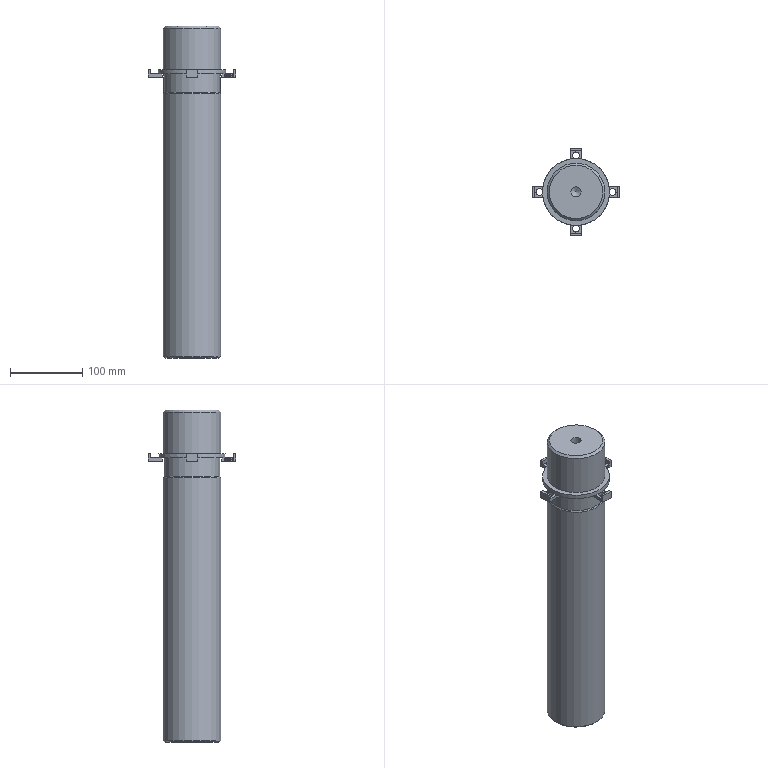Part | STEP file | lll_id2850_x_t | 1 solid | 228 faces | box 121.6 x 121.6 x 460.5 mm | volume 2312756 mm3 | plane 136 | other 76 | cylinder 10 | cone 5 | torus 1 | commonest cylinder face diameters 9 x4 80 x2 8.5 x1 14 x1 78 x1 93 x1